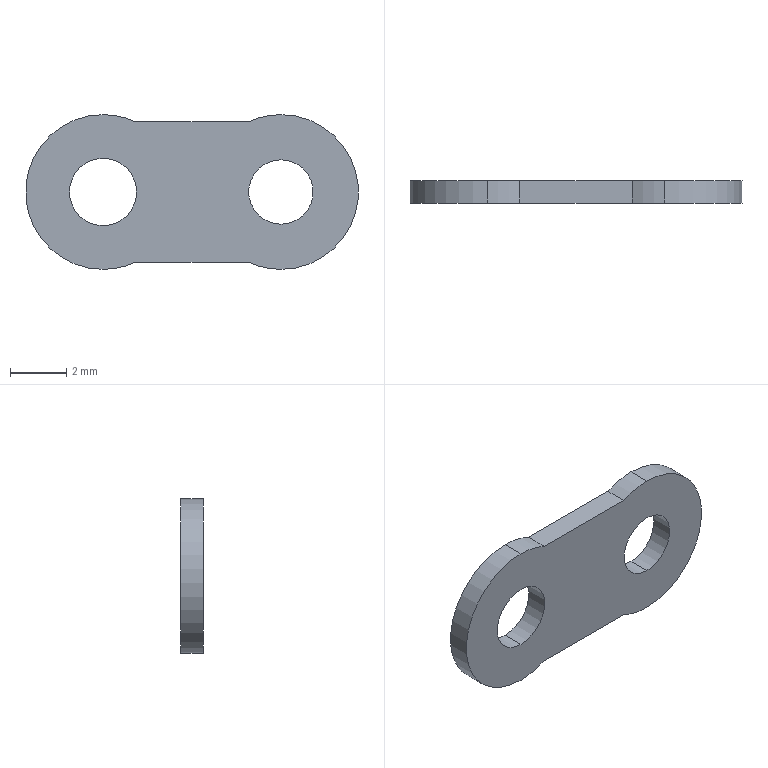Part | SolidWorks | features Extrusion 1 | 1 solid | 14 faces | box 11.87 x 0.8 x 5.52 mm | volume 38.257 mm3 | cylinder 10 | plane 4 | commonest cylinder face diameters 5.52 x6 2.3 x2 2.4 x2
STEP:
#1=CARTESIAN_POINT('',(4.101,0.8,-1.15));
#2=VERTEX_POINT('',#1);
#3=CARTESIAN_POINT('',(4.101,0.8,1.15));
#4=VERTEX_POINT('',#3);
#5=CARTESIAN_POINT('',(4.101,0.8,0.));
#6=DIRECTION('',(0.,1.,0.));
#7=DIRECTION('',(0.,0.,1.));
#8=AXIS2_PLACEMENT_3D('',#5,#6,#7);
#9=CIRCLE('',#8,1.15);
#10=EDGE_CURVE('',#2,#4,#9,.T.);
#11=ORIENTED_EDGE('',*,*,#10,.T.);
#12=CARTESIAN_POINT('',(4.101,0.,1.15));
#13=VERTEX_POINT('',#12);
#14=CARTESIAN_POINT('',(4.101,0.8,1.15));
#15=DIRECTION('',(0.,-1.,0.));
#16=VECTOR('',#15,1000.);
#17=LINE('',#14,#16);
#18=EDGE_CURVE('',#4,#13,#17,.T.);
#19=ORIENTED_EDGE('',*,*,#18,.T.);
#20=CARTESIAN_POINT('',(4.101,0.,-1.15));
#21=VERTEX_POINT('',#20);
#22=CARTESIAN_POINT('',(4.101,0.,0.));
#23=DIRECTION('',(0.,1.,0.));
#24=DIRECTION('',(0.,0.,1.));
#25=AXIS2_PLACEMENT_3D('',#22,#23,#24);
#26=CIRCLE('',#25,1.15);
#27=EDGE_CURVE('',#21,#13,#26,.T.);
#28=ORIENTED_EDGE('',*,*,#27,.F.);
#29=CARTESIAN_POINT('',(4.101,0.8,-1.15));
#30=DIRECTION('',(0.,-1.,0.));
#31=VECTOR('',#30,1000.);
#32=LINE('',#29,#31);
#33=EDGE_CURVE('',#2,#21,#32,.T.);
#34=ORIENTED_EDGE('',*,*,#33,.F.);
#35=EDGE_LOOP('',(#11,#19,#28,#34));
#36=FACE_OUTER_BOUND('',#35,.T.);
#37=CARTESIAN_POINT('',(4.101,0.8,0.));
#38=DIRECTION('',(0.,-1.,0.));
#39=DIRECTION('',(0.,0.,-1.));
#40=AXIS2_PLACEMENT_3D('',#37,#38,#39);
#41=CYLINDRICAL_SURFACE('',#40,1.15);
#42=ADVANCED_FACE('',(#36),#41,.F.);
#43=CARTESIAN_POINT('',(-2.249,0.8,-1.2));
#44=VERTEX_POINT('',#43);
#45=CARTESIAN_POINT('',(-2.249,0.8,1.2));
#46=VERTEX_POINT('',#45);
#47=CARTESIAN_POINT('',(-2.249,0.8,0.));
#48=DIRECTION('',(0.,1.,0.));
#49=DIRECTION('',(0.,0.,1.));
#50=AXIS2_PLACEMENT_3D('',#47,#48,#49);
#51=CIRCLE('',#50,1.2);
#52=EDGE_CURVE('',#44,#46,#51,.T.);
#53=ORIENTED_EDGE('',*,*,#52,.T.);
#54=CARTESIAN_POINT('',(-2.249,0.,1.2));
#55=VERTEX_POINT('',#54);
#56=CARTESIAN_POINT('',(-2.249,0.8,1.2));
#57=DIRECTION('',(0.,-1.,0.));
#58=VECTOR('',#57,1000.);
#59=LINE('',#56,#58);
#60=EDGE_CURVE('',#46,#55,#59,.T.);
#61=ORIENTED_EDGE('',*,*,#60,.T.);
#62=CARTESIAN_POINT('',(-2.249,0.,-1.2));
#63=VERTEX_POINT('',#62);
#64=CARTESIAN_POINT('',(-2.249,0.,0.));
#65=DIRECTION('',(0.,1.,0.));
#66=DIRECTION('',(0.,0.,1.));
#67=AXIS2_PLACEMENT_3D('',#64,#65,#66);
#68=CIRCLE('',#67,1.2);
#69=EDGE_CURVE('',#63,#55,#68,.T.);
#70=ORIENTED_EDGE('',*,*,#69,.F.);
#71=CARTESIAN_POINT('',(-2.249,0.8,-1.2));
#72=DIRECTION('',(0.,-1.,0.));
#73=VECTOR('',#72,1000.);
#74=LINE('',#71,#73);
#75=EDGE_CURVE('',#44,#63,#74,.T.);
#76=ORIENTED_EDGE('',*,*,#75,.F.);
#77=EDGE_LOOP('',(#53,#61,#70,#76));
#78=FACE_OUTER_BOUND('',#77,.T.);
#79=CARTESIAN_POINT('',(-2.249,0.8,0.));
#80=DIRECTION('',(0.,-1.,0.));
#81=DIRECTION('',(0.,0.,-1.));
#82=AXIS2_PLACEMENT_3D('',#79,#80,#81);
#83=CYLINDRICAL_SURFACE('',#82,1.2);
#84=ADVANCED_FACE('',(#78),#83,.F.);
#85=CARTESIAN_POINT('',(4.101,0.8,2.76));
#86=VERTEX_POINT('',#85);
#87=CARTESIAN_POINT('',(4.101,0.8,-2.76));
#88=VERTEX_POINT('',#87);
#89=CARTESIAN_POINT('',(4.101,0.8,0.));
#90=DIRECTION('',(0.,1.,0.));
#91=DIRECTION('',(0.,0.,1.));
#92=AXIS2_PLACEMENT_3D('',#89,#90,#91);
#93=CIRCLE('',#92,2.76);
#94=EDGE_CURVE('',#86,#88,#93,.T.);
#95=ORIENTED_EDGE('',*,*,#94,.F.);
#96=CARTESIAN_POINT('',(4.101,0.,2.76));
#97=VERTEX_POINT('',#96);
#98=CARTESIAN_POINT('',(4.101,0.8,2.76));
#99=DIRECTION('',(0.,-1.,0.));
#100=VECTOR('',#99,1000.);
#101=LINE('',#98,#100);
#102=EDGE_CURVE('',#86,#97,#101,.T.);
#103=ORIENTED_EDGE('',*,*,#102,.T.);
#104=CARTESIAN_POINT('',(4.101,0.,-2.76));
#105=VERTEX_POINT('',#104);
#106=CARTESIAN_POINT('',(4.101,0.,0.));
#107=DIRECTION('',(0.,1.,0.));
#108=DIRECTION('',(0.,0.,1.));
#109=AXIS2_PLACEMENT_3D('',#106,#107,#108);
#110=CIRCLE('',#109,2.76);
#111=EDGE_CURVE('',#97,#105,#110,.T.);
#112=ORIENTED_EDGE('',*,*,#111,.T.);
#113=CARTESIAN_POINT('',(4.101,0.8,-2.76));
#114=DIRECTION('',(0.,-1.,0.));
#115=VECTOR('',#114,1000.);
#116=LINE('',#113,#115);
#117=EDGE_CURVE('',#88,#105,#116,.T.);
#118=ORIENTED_EDGE('',*,*,#117,.F.);
#119=EDGE_LOOP('',(#95,#103,#112,#118));
#120=FACE_OUTER_BOUND('',#119,.T.);
#121=CARTESIAN_POINT('',(4.101,0.8,0.));
#122=DIRECTION('',(0.,-1.,0.));
#123=DIRECTION('',(0.,0.,-1.));
#124=AXIS2_PLACEMENT_3D('',#121,#122,#123);
#125=CYLINDRICAL_SURFACE('',#124,2.76);
#126=ADVANCED_FACE('',(#120),#125,.T.);
#127=CARTESIAN_POINT('',(2.931,0.8,-2.5));
#128=VERTEX_POINT('',#127);
#129=CARTESIAN_POINT('',(4.101,0.8,0.));
#130=DIRECTION('',(0.,1.,0.));
#131=DIRECTION('',(0.,0.,1.));
#132=AXIS2_PLACEMENT_3D('',#129,#130,#131);
#133=CIRCLE('',#132,2.76);
#134=EDGE_CURVE('',#88,#128,#133,.T.);
#135=ORIENTED_EDGE('',*,*,#134,.F.);
#136=ORIENTED_EDGE('',*,*,#117,.T.);
#137=CARTESIAN_POINT('',(2.931,0.,-2.5));
#138=VERTEX_POINT('',#137);
#139=CARTESIAN_POINT('',(4.101,0.,0.));
#140=DIRECTION('',(0.,1.,0.));
#141=DIRECTION('',(0.,0.,1.));
#142=AXIS2_PLACEMENT_3D('',#139,#140,#141);
#143=CIRCLE('',#142,2.76);
#144=EDGE_CURVE('',#105,#138,#143,.T.);
#145=ORIENTED_EDGE('',*,*,#144,.T.);
#146=CARTESIAN_POINT('',(2.931,0.8,-2.5));
#147=DIRECTION('',(0.,-1.,0.));
#148=VECTOR('',#147,1000.);
#149=LINE('',#146,#148);
#150=EDGE_CURVE('',#128,#138,#149,.T.);
#151=ORIENTED_EDGE('',*,*,#150,.F.);
#152=EDGE_LOOP('',(#135,#136,#145,#151));
#153=FACE_OUTER_BOUND('',#152,.T.);
#154=CARTESIAN_POINT('',(4.101,0.8,0.));
#155=DIRECTION('',(0.,-1.,0.));
#156=DIRECTION('',(0.,0.,-1.));
#157=AXIS2_PLACEMENT_3D('',#154,#155,#156);
#158=CYLINDRICAL_SURFACE('',#157,2.76);
#159=ADVANCED_FACE('',(#153),#158,.T.);
#160=CARTESIAN_POINT('',(-2.249,0.8,2.76));
#161=VERTEX_POINT('',#160);
#162=CARTESIAN_POINT('',(-1.08,0.8,2.5));
#163=VERTEX_POINT('',#162);
#164=CARTESIAN_POINT('',(-2.249,0.8,0.));
#165=DIRECTION('',(0.,1.,0.));
#166=DIRECTION('',(0.,0.,1.));
#167=AXIS2_PLACEMENT_3D('',#164,#165,#166);
#168=CIRCLE('',#167,2.76);
#169=EDGE_CURVE('',#161,#163,#168,.T.);
#170=ORIENTED_EDGE('',*,*,#169,.F.);
#171=CARTESIAN_POINT('',(-2.249,0.,2.76));
#172=VERTEX_POINT('',#171);
#173=CARTESIAN_POINT('',(-2.249,0.8,2.76));
#174=DIRECTION('',(0.,-1.,0.));
#175=VECTOR('',#174,1000.);
#176=LINE('',#173,#175);
#177=EDGE_CURVE('',#161,#172,#176,.T.);
#178=ORIENTED_EDGE('',*,*,#177,.T.);
#179=CARTESIAN_POINT('',(-1.08,0.,2.5));
#180=VERTEX_POINT('',#179);
#181=CARTESIAN_POINT('',(-2.249,0.,0.));
#182=DIRECTION('',(0.,1.,0.));
#183=DIRECTION('',(0.,0.,1.));
#184=AXIS2_PLACEMENT_3D('',#181,#182,#183);
#185=CIRCLE('',#184,2.76);
#186=EDGE_CURVE('',#172,#180,#185,.T.);
#187=ORIENTED_EDGE('',*,*,#186,.T.);
#188=CARTESIAN_POINT('',(-1.08,0.8,2.5));
#189=DIRECTION('',(0.,-1.,0.));
#190=VECTOR('',#189,1000.);
#191=LINE('',#188,#190);
#192=EDGE_CURVE('',#163,#180,#191,.T.);
#193=ORIENTED_EDGE('',*,*,#192,.F.);
#194=EDGE_LOOP('',(#170,#178,#187,#193));
#195=FACE_OUTER_BOUND('',#194,.T.);
#196=CARTESIAN_POINT('',(-2.249,0.8,0.));
#197=DIRECTION('',(0.,-1.,0.));
#198=DIRECTION('',(0.,0.,-1.));
#199=AXIS2_PLACEMENT_3D('',#196,#197,#198);
#200=CYLINDRICAL_SURFACE('',#199,2.76);
#201=ADVANCED_FACE('',(#195),#200,.T.);
#202=ORIENTED_EDGE('',*,*,#177,.F.);
#203=CARTESIAN_POINT('',(-2.249,0.8,-2.76));
#204=VERTEX_POINT('',#203);
#205=CARTESIAN_POINT('',(-2.249,0.8,0.));
#206=DIRECTION('',(0.,1.,0.));
#207=DIRECTION('',(0.,0.,1.));
#208=AXIS2_PLACEMENT_3D('',#205,#206,#207);
#209=CIRCLE('',#208,2.76);
#210=EDGE_CURVE('',#204,#161,#209,.T.);
#211=ORIENTED_EDGE('',*,*,#210,.F.);
#212=CARTESIAN_POINT('',(-2.249,0.,-2.76));
#213=VERTEX_POINT('',#212);
#214=CARTESIAN_POINT('',(-2.249,0.8,-2.76));
#215=DIRECTION('',(0.,-1.,0.));
#216=VECTOR('',#215,1000.);
#217=LINE('',#214,#216);
#218=EDGE_CURVE('',#204,#213,#217,.T.);
#219=ORIENTED_EDGE('',*,*,#218,.T.);
#220=CARTESIAN_POINT('',(-2.249,0.,0.));
#221=DIRECTION('',(0.,1.,0.));
#222=DIRECTION('',(0.,0.,1.));
#223=AXIS2_PLACEMENT_3D('',#220,#221,#222);
#224=CIRCLE('',#223,2.76);
#225=EDGE_CURVE('',#213,#172,#224,.T.);
#226=ORIENTED_EDGE('',*,*,#225,.T.);
#227=EDGE_LOOP('',(#202,#211,#219,#226));
#228=FACE_OUTER_BOUND('',#227,.T.);
#229=CARTESIAN_POINT('',(-2.249,0.8,0.));
#230=DIRECTION('',(0.,-1.,0.));
#231=DIRECTION('',(0.,0.,-1.));
#232=AXIS2_PLACEMENT_3D('',#229,#230,#231);
#233=CYLINDRICAL_SURFACE('',#232,2.76);
#234=ADVANCED_FACE('',(#228),#233,.T.);
#235=ORIENTED_EDGE('',*,*,#52,.F.);
#236=CARTESIAN_POINT('',(-2.249,0.8,0.));
#237=DIRECTION('',(0.,1.,0.));
#238=DIRECTION('',(0.,0.,1.));
#239=AXIS2_PLACEMENT_3D('',#236,#237,#238);
#240=CIRCLE('',#239,1.2);
#241=EDGE_CURVE('',#46,#44,#240,.T.);
#242=ORIENTED_EDGE('',*,*,#241,.F.);
#243=EDGE_LOOP('',(#235,#242));
#244=FACE_BOUND('',#243,.T.);
#245=CARTESIAN_POINT('',(-1.08,0.8,-2.5));
#246=VERTEX_POINT('',#245);
#247=CARTESIAN_POINT('',(-2.249,0.8,0.));
#248=DIRECTION('',(0.,1.,0.));
#249=DIRECTION('',(0.,0.,1.));
#250=AXIS2_PLACEMENT_3D('',#247,#248,#249);
#251=CIRCLE('',#250,2.76);
#252=EDGE_CURVE('',#246,#204,#251,.T.);
#253=ORIENTED_EDGE('',*,*,#252,.T.);
#254=ORIENTED_EDGE('',*,*,#210,.T.);
#255=ORIENTED_EDGE('',*,*,#169,.T.);
#256=CARTESIAN_POINT('',(2.931,0.8,2.5));
#257=VERTEX_POINT('',#256);
#258=CARTESIAN_POINT('',(-1.08,0.8,2.5));
#259=DIRECTION('',(1.,0.,0.));
#260=VECTOR('',#259,1000.);
#261=LINE('',#258,#260);
#262=EDGE_CURVE('',#163,#257,#261,.T.);
#263=ORIENTED_EDGE('',*,*,#262,.T.);
#264=CARTESIAN_POINT('',(4.101,0.8,0.));
#265=DIRECTION('',(0.,1.,0.));
#266=DIRECTION('',(0.,0.,1.));
#267=AXIS2_PLACEMENT_3D('',#264,#265,#266);
#268=CIRCLE('',#267,2.76);
#269=EDGE_CURVE('',#257,#86,#268,.T.);
#270=ORIENTED_EDGE('',*,*,#269,.T.);
#271=ORIENTED_EDGE('',*,*,#94,.T.);
#272=ORIENTED_EDGE('',*,*,#134,.T.);
#273=CARTESIAN_POINT('',(-1.08,0.8,-2.5));
#274=DIRECTION('',(-1.,0.,0.));
#275=VECTOR('',#274,1000.);
#276=LINE('',#273,#275);
#277=EDGE_CURVE('',#128,#246,#276,.T.);
#278=ORIENTED_EDGE('',*,*,#277,.T.);
#279=EDGE_LOOP('',(#253,#254,#255,#263,#270,#271,#272,#278));
#280=FACE_OUTER_BOUND('',#279,.T.);
#281=ORIENTED_EDGE('',*,*,#10,.F.);
#282=CARTESIAN_POINT('',(4.101,0.8,0.));
#283=DIRECTION('',(0.,1.,0.));
#284=DIRECTION('',(0.,0.,1.));
#285=AXIS2_PLACEMENT_3D('',#282,#283,#284);
#286=CIRCLE('',#285,1.15);
#287=EDGE_CURVE('',#4,#2,#286,.T.);
#288=ORIENTED_EDGE('',*,*,#287,.F.);
#289=EDGE_LOOP('',(#281,#288));
#290=FACE_BOUND('',#289,.T.);
#291=CARTESIAN_POINT('',(-2.249,0.8,0.));
#292=DIRECTION('',(0.,1.,0.));
#293=DIRECTION('',(0.,0.,1.));
#294=AXIS2_PLACEMENT_3D('',#291,#292,#293);
#295=PLANE('',#294);
#296=ADVANCED_FACE('',(#244,#280,#290),#295,.T.);
#297=CARTESIAN_POINT('',(-1.08,0.,-2.5));
#298=VERTEX_POINT('',#297);
#299=CARTESIAN_POINT('',(-2.249,0.,0.));
#300=DIRECTION('',(0.,1.,0.));
#301=DIRECTION('',(0.,0.,1.));
#302=AXIS2_PLACEMENT_3D('',#299,#300,#301);
#303=CIRCLE('',#302,2.76);
#304=EDGE_CURVE('',#298,#213,#303,.T.);
#305=ORIENTED_EDGE('',*,*,#304,.F.);
#306=CARTESIAN_POINT('',(-1.08,0.,-2.5));
#307=DIRECTION('',(-1.,0.,0.));
#308=VECTOR('',#307,1000.);
#309=LINE('',#306,#308);
#310=EDGE_CURVE('',#138,#298,#309,.T.);
#311=ORIENTED_EDGE('',*,*,#310,.F.);
#312=ORIENTED_EDGE('',*,*,#144,.F.);
#313=ORIENTED_EDGE('',*,*,#111,.F.);
#314=CARTESIAN_POINT('',(2.931,0.,2.5));
#315=VERTEX_POINT('',#314);
#316=CARTESIAN_POINT('',(4.101,0.,0.));
#317=DIRECTION('',(0.,1.,0.));
#318=DIRECTION('',(0.,0.,1.));
#319=AXIS2_PLACEMENT_3D('',#316,#317,#318);
#320=CIRCLE('',#319,2.76);
#321=EDGE_CURVE('',#315,#97,#320,.T.);
#322=ORIENTED_EDGE('',*,*,#321,.F.);
#323=CARTESIAN_POINT('',(-1.08,0.,2.5));
#324=DIRECTION('',(1.,0.,0.));
#325=VECTOR('',#324,1000.);
#326=LINE('',#323,#325);
#327=EDGE_CURVE('',#180,#315,#326,.T.);
#328=ORIENTED_EDGE('',*,*,#327,.F.);
#329=ORIENTED_EDGE('',*,*,#186,.F.);
#330=ORIENTED_EDGE('',*,*,#225,.F.);
#331=EDGE_LOOP('',(#305,#311,#312,#313,#322,#328,#329,#330));
#332=FACE_OUTER_BOUND('',#331,.T.);
#333=ORIENTED_EDGE('',*,*,#69,.T.);
#334=CARTESIAN_POINT('',(-2.249,0.,0.));
#335=DIRECTION('',(0.,1.,0.));
#336=DIRECTION('',(0.,0.,1.));
#337=AXIS2_PLACEMENT_3D('',#334,#335,#336);
#338=CIRCLE('',#337,1.2);
#339=EDGE_CURVE('',#55,#63,#338,.T.);
#340=ORIENTED_EDGE('',*,*,#339,.T.);
#341=EDGE_LOOP('',(#333,#340));
#342=FACE_BOUND('',#341,.T.);
#343=ORIENTED_EDGE('',*,*,#27,.T.);
#344=CARTESIAN_POINT('',(4.101,0.,0.));
#345=DIRECTION('',(0.,1.,0.));
#346=DIRECTION('',(0.,0.,1.));
#347=AXIS2_PLACEMENT_3D('',#344,#345,#346);
#348=CIRCLE('',#347,1.15);
#349=EDGE_CURVE('',#13,#21,#348,.T.);
#350=ORIENTED_EDGE('',*,*,#349,.T.);
#351=EDGE_LOOP('',(#343,#350));
#352=FACE_BOUND('',#351,.T.);
#353=CARTESIAN_POINT('',(-2.249,0.,0.));
#354=DIRECTION('',(0.,1.,0.));
#355=DIRECTION('',(0.,0.,1.));
#356=AXIS2_PLACEMENT_3D('',#353,#354,#355);
#357=PLANE('',#356);
#358=ADVANCED_FACE('',(#332,#342,#352),#357,.F.);
#359=ORIENTED_EDGE('',*,*,#218,.F.);
#360=ORIENTED_EDGE('',*,*,#252,.F.);
#361=CARTESIAN_POINT('',(-1.08,0.8,-2.5));
#362=DIRECTION('',(0.,-1.,0.));
#363=VECTOR('',#362,1000.);
#364=LINE('',#361,#363);
#365=EDGE_CURVE('',#246,#298,#364,.T.);
#366=ORIENTED_EDGE('',*,*,#365,.T.);
#367=ORIENTED_EDGE('',*,*,#304,.T.);
#368=EDGE_LOOP('',(#359,#360,#366,#367));
#369=FACE_OUTER_BOUND('',#368,.T.);
#370=CARTESIAN_POINT('',(-2.249,0.8,0.));
#371=DIRECTION('',(0.,-1.,0.));
#372=DIRECTION('',(0.,0.,-1.));
#373=AXIS2_PLACEMENT_3D('',#370,#371,#372);
#374=CYLINDRICAL_SURFACE('',#373,2.76);
#375=ADVANCED_FACE('',(#369),#374,.T.);
#376=ORIENTED_EDGE('',*,*,#327,.T.);
#377=CARTESIAN_POINT('',(2.931,0.8,2.5));
#378=DIRECTION('',(0.,-1.,0.));
#379=VECTOR('',#378,1000.);
#380=LINE('',#377,#379);
#381=EDGE_CURVE('',#257,#315,#380,.T.);
#382=ORIENTED_EDGE('',*,*,#381,.F.);
#383=ORIENTED_EDGE('',*,*,#262,.F.);
#384=ORIENTED_EDGE('',*,*,#192,.T.);
#385=EDGE_LOOP('',(#376,#382,#383,#384));
#386=FACE_OUTER_BOUND('',#385,.T.);
#387=CARTESIAN_POINT('',(-1.08,0.8,2.5));
#388=DIRECTION('',(0.,0.,-1.));
#389=DIRECTION('',(-1.,0.,0.));
#390=AXIS2_PLACEMENT_3D('',#387,#388,#389);
#391=PLANE('',#390);
#392=ADVANCED_FACE('',(#386),#391,.F.);
#393=ORIENTED_EDGE('',*,*,#102,.F.);
#394=ORIENTED_EDGE('',*,*,#269,.F.);
#395=ORIENTED_EDGE('',*,*,#381,.T.);
#396=ORIENTED_EDGE('',*,*,#321,.T.);
#397=EDGE_LOOP('',(#393,#394,#395,#396));
#398=FACE_OUTER_BOUND('',#397,.T.);
#399=CARTESIAN_POINT('',(4.101,0.8,0.));
#400=DIRECTION('',(0.,-1.,0.));
#401=DIRECTION('',(0.,0.,-1.));
#402=AXIS2_PLACEMENT_3D('',#399,#400,#401);
#403=CYLINDRICAL_SURFACE('',#402,2.76);
#404=ADVANCED_FACE('',(#398),#403,.T.);
#405=ORIENTED_EDGE('',*,*,#310,.T.);
#406=ORIENTED_EDGE('',*,*,#365,.F.);
#407=ORIENTED_EDGE('',*,*,#277,.F.);
#408=ORIENTED_EDGE('',*,*,#150,.T.);
#409=EDGE_LOOP('',(#405,#406,#407,#408));
#410=FACE_OUTER_BOUND('',#409,.T.);
#411=CARTESIAN_POINT('',(-1.08,0.8,-2.5));
#412=DIRECTION('',(0.,0.,1.));
#413=DIRECTION('',(1.,0.,0.));
#414=AXIS2_PLACEMENT_3D('',#411,#412,#413);
#415=PLANE('',#414);
#416=ADVANCED_FACE('',(#410),#415,.F.);
#417=ORIENTED_EDGE('',*,*,#60,.F.);
#418=ORIENTED_EDGE('',*,*,#241,.T.);
#419=ORIENTED_EDGE('',*,*,#75,.T.);
#420=ORIENTED_EDGE('',*,*,#339,.F.);
#421=EDGE_LOOP('',(#417,#418,#419,#420));
#422=FACE_OUTER_BOUND('',#421,.T.);
#423=CARTESIAN_POINT('',(-2.249,0.8,0.));
#424=DIRECTION('',(0.,-1.,0.));
#425=DIRECTION('',(0.,0.,-1.));
#426=AXIS2_PLACEMENT_3D('',#423,#424,#425);
#427=CYLINDRICAL_SURFACE('',#426,1.2);
#428=ADVANCED_FACE('',(#422),#427,.F.);
#429=ORIENTED_EDGE('',*,*,#18,.F.);
#430=ORIENTED_EDGE('',*,*,#287,.T.);
#431=ORIENTED_EDGE('',*,*,#33,.T.);
#432=ORIENTED_EDGE('',*,*,#349,.F.);
#433=EDGE_LOOP('',(#429,#430,#431,#432));
#434=FACE_OUTER_BOUND('',#433,.T.);
#435=CARTESIAN_POINT('',(4.101,0.8,0.));
#436=DIRECTION('',(0.,-1.,0.));
#437=DIRECTION('',(0.,0.,-1.));
#438=AXIS2_PLACEMENT_3D('',#435,#436,#437);
#439=CYLINDRICAL_SURFACE('',#438,1.15);
#440=ADVANCED_FACE('',(#434),#439,.F.);
#441=CLOSED_SHELL('',(#42,#84,#126,#159,#201,#234,#296,#358,#375,#392,#404,#416,#428,#440));
#442=MANIFOLD_SOLID_BREP('',#441);
#443=CARTESIAN_POINT('',(0.,0.,0.));
#444=DIRECTION('',(0.,0.,1.));
#445=DIRECTION('',(1.,0.,0.));
#446=AXIS2_PLACEMENT_3D('',#443,#444,#445);
#447=(LENGTH_UNIT()NAMED_UNIT(*)SI_UNIT(.MILLI.,.METRE.));
#448=UNCERTAINTY_MEASURE_WITH_UNIT(LENGTH_MEASURE(0.00001),#447,'','');
#449=(NAMED_UNIT(*)PLANE_ANGLE_UNIT()SI_UNIT($,.RADIAN.));
#450=(NAMED_UNIT(*)SI_UNIT($,.STERADIAN.)SOLID_ANGLE_UNIT());
#451=(GEOMETRIC_REPRESENTATION_CONTEXT(3)GLOBAL_UNCERTAINTY_ASSIGNED_CONTEXT((#448))GLOBAL_UNIT_ASSIGNED_CONTEXT((#447,#449,#450))REPRESENTATION_CONTEXT('',''));
#452=ADVANCED_BREP_SHAPE_REPRESENTATION('',(#442,#446),#451);